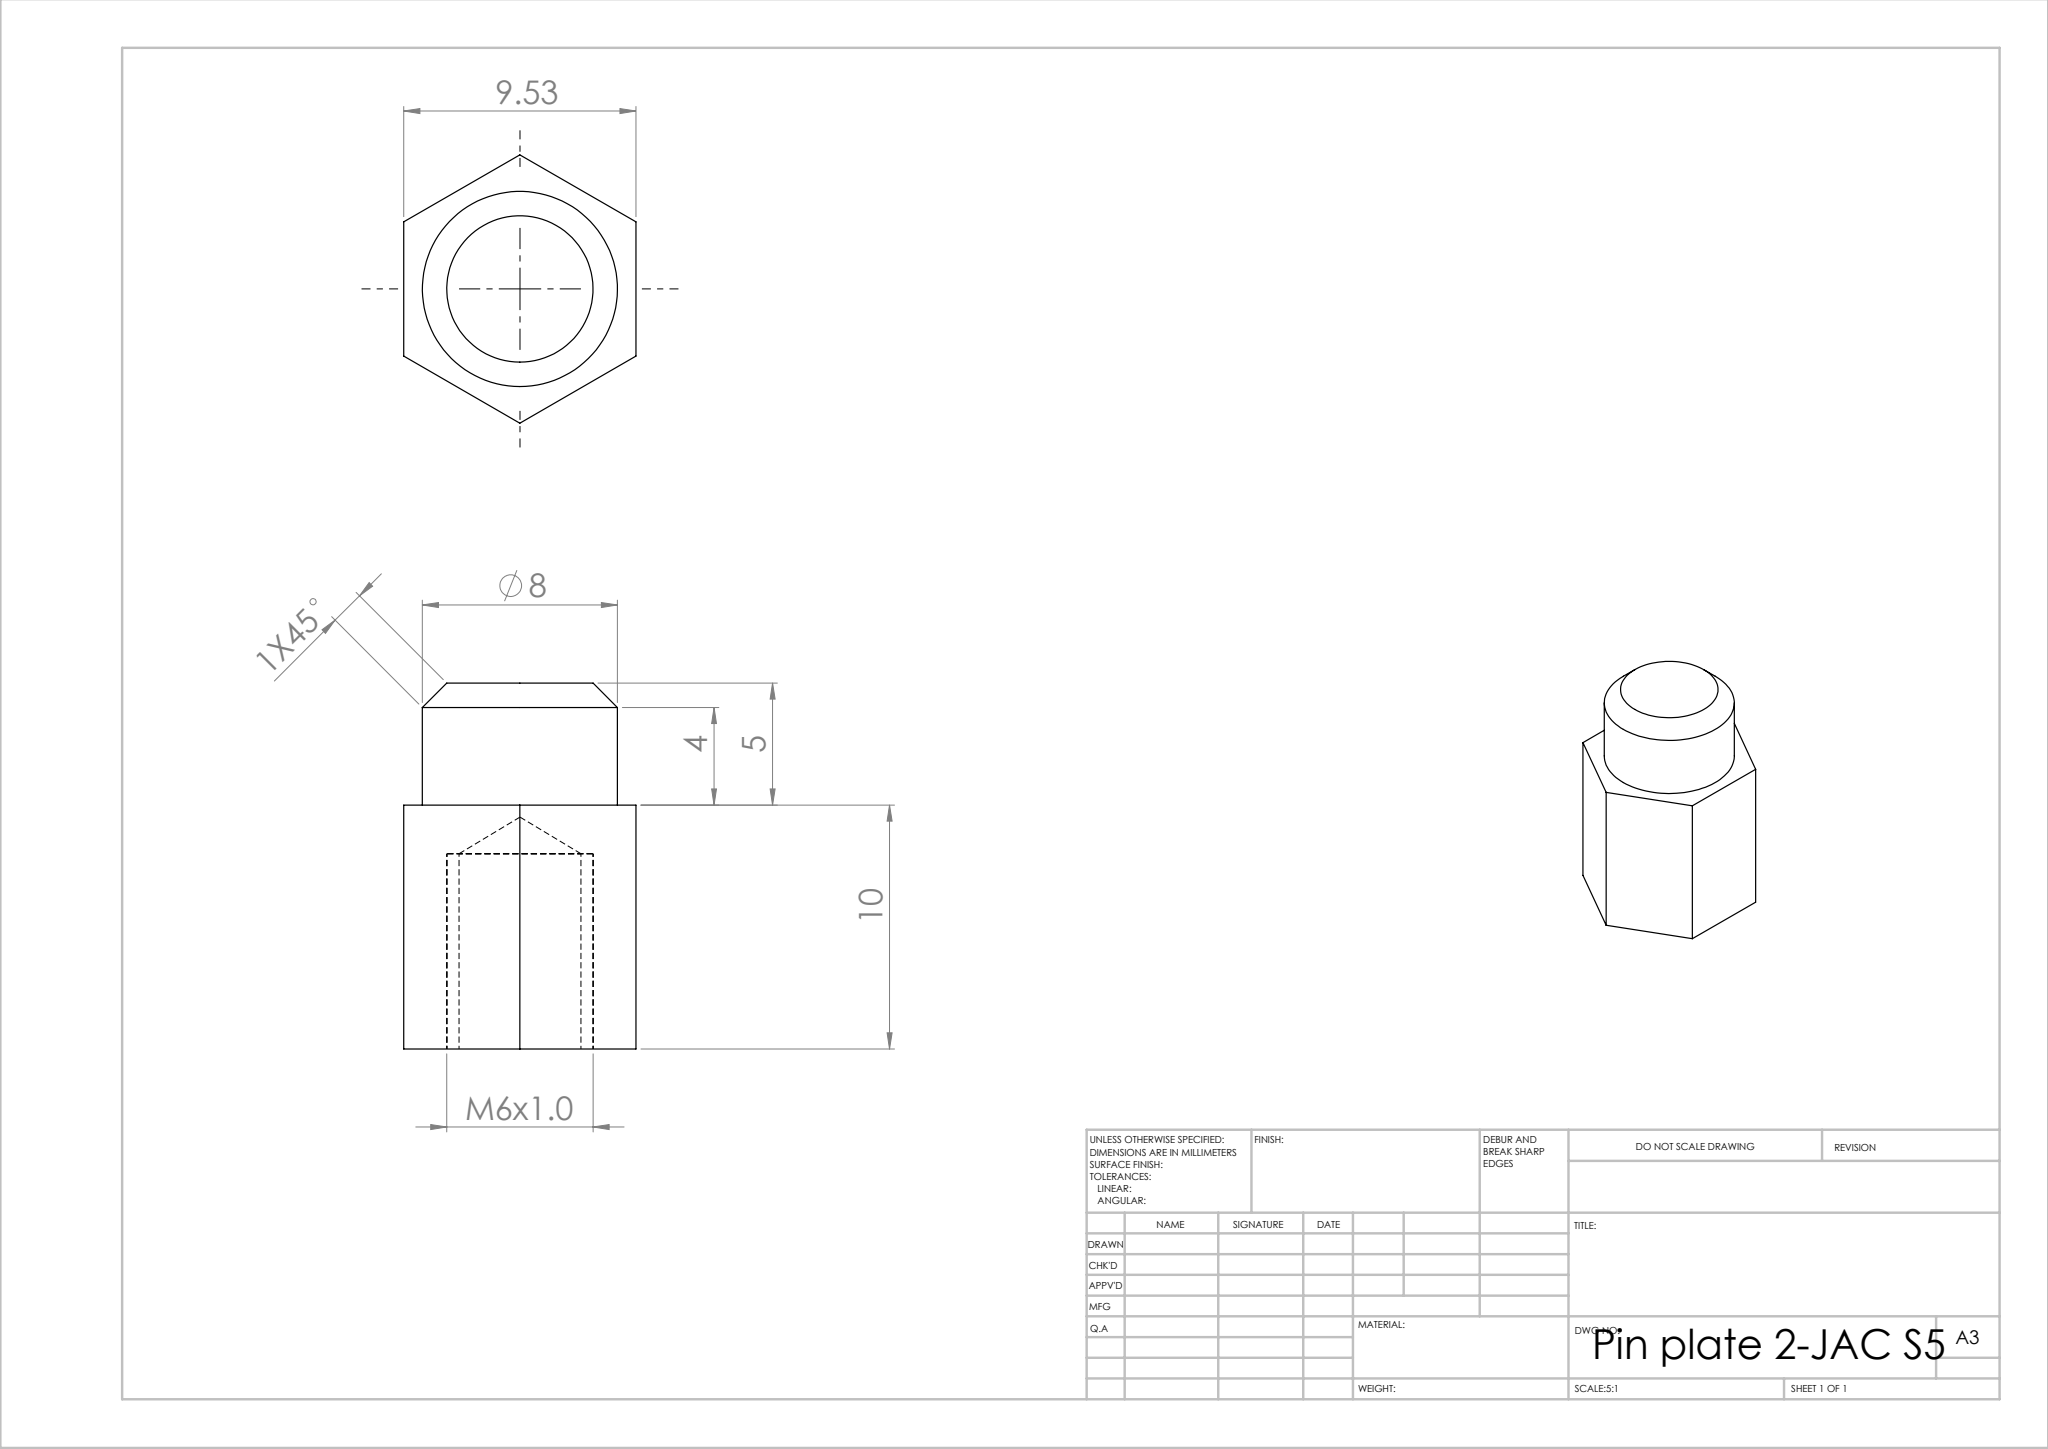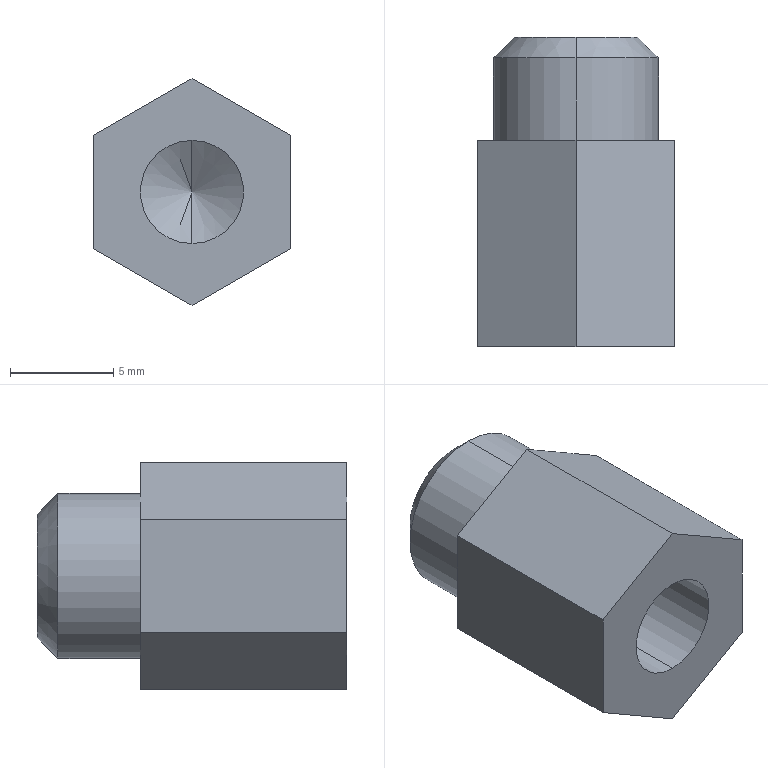Part | SolidWorks | features 3DProfileFeature 1, Chamfer 1, Extrusion 1, HoleWzd 1, ICE 1 | 1 solid | 17 faces | box 9.526 x 15 x 11 mm | volume 858.815 mm3 | plane 9 | cylinder 4 | cone 4 | commonest cylinder face diameters 5 x2 8 x2